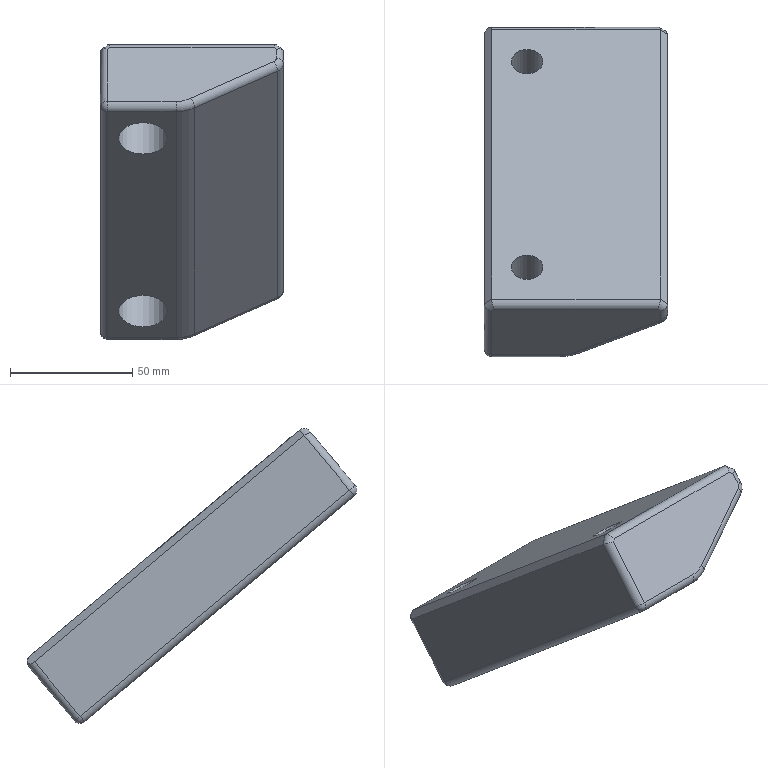Part | NX | features MAIN_BODY 2 | 1 solid | 37 faces | box 75 x 134.951 x 120.777 mm | volume 305128 mm3 | cylinder 20 | plane 11 | torus 4 | sphere 2 | commonest cylinder face diameters 6 x14 13 x2 20 x2 10 x1 30 x1
STEP:
#1=CARTESIAN_POINT('',(-217.5,186.664,-117.468));
#2=VERTEX_POINT('',#1);
#3=CARTESIAN_POINT('',(-217.5,191.644,-121.646));
#4=DIRECTION('',(0.,0.6428,0.766));
#5=DIRECTION('',(0.,-0.766,0.6428));
#6=AXIS2_PLACEMENT_3D('',#3,#4,#5);
#7=CIRCLE('',#6,6.5);
#8=EDGE_CURVE('',#2,#2,#7,.T.);
#9=ORIENTED_EDGE('',*,*,#8,.T.);
#10=EDGE_LOOP('',(#9));
#11=FACE_BOUND('',#10,.T.);
#12=CARTESIAN_POINT('',(-217.5,183.983,-115.218));
#13=VERTEX_POINT('',#12);
#14=CARTESIAN_POINT('',(-217.5,191.644,-121.646));
#15=DIRECTION('',(0.,0.6428,0.766));
#16=DIRECTION('',(0.,-0.766,0.6428));
#17=AXIS2_PLACEMENT_3D('',#14,#15,#16);
#18=CIRCLE('',#17,10.);
#19=EDGE_CURVE('',#13,#13,#18,.T.);
#20=ORIENTED_EDGE('',*,*,#19,.F.);
#21=EDGE_LOOP('',(#20));
#22=FACE_BOUND('',#21,.T.);
#23=CARTESIAN_POINT('',(-217.5,191.644,-121.646));
#24=DIRECTION('',(0.,0.6428,0.766));
#25=DIRECTION('',(0.,-0.766,0.6428));
#26=AXIS2_PLACEMENT_3D('',#23,#24,#25);
#27=PLANE('',#26);
#28=ADVANCED_FACE('',(#11,#22),#27,.F.);
#29=CARTESIAN_POINT('',(-163.,183.237,-100.55));
#30=VERTEX_POINT('',#29);
#31=CARTESIAN_POINT('',(-164.243,184.036,-99.598));
#32=VERTEX_POINT('',#31);
#33=CARTESIAN_POINT('',(-133.621,164.353,-123.055));
#34=DIRECTION('',(-0.7071,0.4545,0.5417));
#35=VECTOR('',#34,1000.);
#36=LINE('',#33,#35);
#37=EDGE_CURVE('',#30,#32,#36,.T.);
#38=ORIENTED_EDGE('',*,*,#37,.T.);
#39=CARTESIAN_POINT('',(-230.757,184.036,-99.598));
#40=VERTEX_POINT('',#39);
#41=CARTESIAN_POINT('',(-135.,184.036,-99.598));
#42=DIRECTION('',(-1.,0.,0.));
#43=VECTOR('',#42,1000.);
#44=LINE('',#41,#43);
#45=EDGE_CURVE('',#32,#40,#44,.T.);
#46=ORIENTED_EDGE('',*,*,#45,.T.);
#47=CARTESIAN_POINT('',(-232.,183.237,-100.55));
#48=VERTEX_POINT('',#47);
#49=CARTESIAN_POINT('',(-198.879,204.527,-75.177));
#50=DIRECTION('',(0.7071,0.4545,0.5417));
#51=VECTOR('',#50,1000.);
#52=LINE('',#49,#51);
#53=EDGE_CURVE('',#40,#48,#52,.F.);
#54=ORIENTED_EDGE('',*,*,#53,.T.);
#55=CARTESIAN_POINT('',(-232.,165.395,-121.813));
#56=VERTEX_POINT('',#55);
#57=CARTESIAN_POINT('',(-232.,163.467,-124.111));
#58=DIRECTION('',(0.,-0.6428,-0.766));
#59=VECTOR('',#58,1000.);
#60=LINE('',#57,#59);
#61=EDGE_CURVE('',#48,#56,#60,.T.);
#62=ORIENTED_EDGE('',*,*,#61,.T.);
#63=CARTESIAN_POINT('',(-204.019,165.395,-121.813));
#64=VERTEX_POINT('',#63);
#65=CARTESIAN_POINT('',(-135.,165.395,-121.813));
#66=DIRECTION('',(-1.,0.,0.));
#67=VECTOR('',#66,1000.);
#68=LINE('',#65,#67);
#69=EDGE_CURVE('',#56,#64,#68,.F.);
#70=ORIENTED_EDGE('',*,*,#69,.T.);
#71=CARTESIAN_POINT('',(-198.019,166.429,-120.581));
#72=VERTEX_POINT('',#71);
#73=CARTESIAN_POINT('',(-204.019,173.109,-112.62));
#74=DIRECTION('',(0.,-0.766,0.6428));
#75=DIRECTION('',(0.,-0.6428,-0.766));
#76=AXIS2_PLACEMENT_3D('',#73,#74,#75);
#77=CIRCLE('',#76,12.);
#78=EDGE_CURVE('',#64,#72,#77,.T.);
#79=ORIENTED_EDGE('',*,*,#78,.T.);
#80=CARTESIAN_POINT('',(-164.,179.054,-105.535));
#81=VERTEX_POINT('',#80);
#82=CARTESIAN_POINT('',(-152.75,183.229,-100.56));
#83=DIRECTION('',(0.866,0.3214,0.383));
#84=VECTOR('',#83,1000.);
#85=LINE('',#82,#84);
#86=EDGE_CURVE('',#72,#81,#85,.T.);
#87=ORIENTED_EDGE('',*,*,#86,.T.);
#88=CARTESIAN_POINT('',(-163.,180.167,-104.209));
#89=VERTEX_POINT('',#88);
#90=CARTESIAN_POINT('',(-165.,180.167,-104.209));
#91=DIRECTION('',(0.,-0.766,0.6428));
#92=DIRECTION('',(0.,-0.6428,-0.766));
#93=AXIS2_PLACEMENT_3D('',#90,#91,#92);
#94=CIRCLE('',#93,2.);
#95=EDGE_CURVE('',#81,#89,#94,.T.);
#96=ORIENTED_EDGE('',*,*,#95,.T.);
#97=CARTESIAN_POINT('',(-163.,184.036,-99.598));
#98=DIRECTION('',(0.,0.6428,0.766));
#99=VECTOR('',#98,1000.);
#100=LINE('',#97,#99);
#101=EDGE_CURVE('',#89,#30,#100,.T.);
#102=ORIENTED_EDGE('',*,*,#101,.T.);
#103=EDGE_LOOP('',(#38,#46,#54,#62,#70,#79,#87,#96,#102));
#104=FACE_BOUND('',#103,.T.);
#105=CARTESIAN_POINT('',(-135.,163.467,-124.111));
#106=DIRECTION('',(0.,-0.766,0.6428));
#107=DIRECTION('',(-1.,0.,0.));
#108=AXIS2_PLACEMENT_3D('',#105,#106,#107);
#109=PLANE('',#108);
#110=ADVANCED_FACE('',(#104),#109,.T.);
#111=CARTESIAN_POINT('',(-160.,182.465,-106.137));
#112=VERTEX_POINT('',#111);
#113=CARTESIAN_POINT('',(-163.,182.465,-106.137));
#114=DIRECTION('',(0.,-0.6428,-0.766));
#115=DIRECTION('',(0.,0.766,-0.6428));
#116=AXIS2_PLACEMENT_3D('',#113,#114,#115);
#117=CIRCLE('',#116,3.);
#118=EDGE_CURVE('',#112,#89,#117,.T.);
#119=ORIENTED_EDGE('',*,*,#118,.F.);
#120=CARTESIAN_POINT('',(-160.,186.334,-101.526));
#121=VERTEX_POINT('',#120);
#122=CARTESIAN_POINT('',(-160.,182.465,-106.137));
#123=DIRECTION('',(0.,0.6428,0.766));
#124=VECTOR('',#123,1000.);
#125=LINE('',#122,#124);
#126=EDGE_CURVE('',#121,#112,#125,.F.);
#127=ORIENTED_EDGE('',*,*,#126,.F.);
#128=CARTESIAN_POINT('',(-163.,185.536,-102.478));
#129=DIRECTION('',(0.3827,-0.5939,-0.7077));
#130=DIRECTION('',(-0.9239,-0.246,-0.2932));
#131=AXIS2_PLACEMENT_3D('',#128,#129,#130);
#132=ELLIPSE('',#131,3.247,3.);
#133=EDGE_CURVE('',#30,#121,#132,.F.);
#134=ORIENTED_EDGE('',*,*,#133,.F.);
#135=ORIENTED_EDGE('',*,*,#101,.F.);
#136=EDGE_LOOP('',(#119,#127,#134,#135));
#137=FACE_BOUND('',#136,.T.);
#138=CARTESIAN_POINT('',(-163.,165.765,-126.039));
#139=DIRECTION('',(0.,-0.6428,-0.766));
#140=DIRECTION('',(0.,0.766,-0.6428));
#141=AXIS2_PLACEMENT_3D('',#138,#139,#140);
#142=CYLINDRICAL_SURFACE('',#141,3.);
#143=ADVANCED_FACE('',(#137),#142,.T.);
#144=CARTESIAN_POINT('',(-204.019,165.765,-126.039));
#145=VERTEX_POINT('',#144);
#146=CARTESIAN_POINT('',(-204.019,167.693,-123.741));
#147=DIRECTION('',(-1.,0.,0.));
#148=DIRECTION('',(0.,0.9063,0.4226));
#149=AXIS2_PLACEMENT_3D('',#146,#147,#148);
#150=CIRCLE('',#149,3.);
#151=EDGE_CURVE('',#145,#64,#150,.T.);
#152=ORIENTED_EDGE('',*,*,#151,.T.);
#153=ORIENTED_EDGE('',*,*,#69,.F.);
#154=CARTESIAN_POINT('',(-232.,165.765,-126.039));
#155=VERTEX_POINT('',#154);
#156=CARTESIAN_POINT('',(-232.,167.693,-123.741));
#157=DIRECTION('',(-1.,0.,0.));
#158=DIRECTION('',(0.,0.9063,0.4226));
#159=AXIS2_PLACEMENT_3D('',#156,#157,#158);
#160=CIRCLE('',#159,3.);
#161=EDGE_CURVE('',#155,#56,#160,.T.);
#162=ORIENTED_EDGE('',*,*,#161,.F.);
#163=CARTESIAN_POINT('',(-285.,165.765,-126.039));
#164=DIRECTION('',(-1.,0.,0.));
#165=VECTOR('',#164,1000.);
#166=LINE('',#163,#165);
#167=EDGE_CURVE('',#145,#155,#166,.T.);
#168=ORIENTED_EDGE('',*,*,#167,.F.);
#169=EDGE_LOOP('',(#152,#153,#162,#168));
#170=FACE_BOUND('',#169,.T.);
#171=CARTESIAN_POINT('',(-285.,167.693,-123.741));
#172=DIRECTION('',(-1.,0.,0.));
#173=DIRECTION('',(0.,0.4226,-0.9063));
#174=AXIS2_PLACEMENT_3D('',#171,#172,#173);
#175=CYLINDRICAL_SURFACE('',#174,3.);
#176=ADVANCED_FACE('',(#170),#175,.T.);
#177=ORIENTED_EDGE('',*,*,#19,.T.);
#178=EDGE_LOOP('',(#177));
#179=FACE_BOUND('',#178,.T.);
#180=CARTESIAN_POINT('',(-217.5,171.127,-130.539));
#181=VERTEX_POINT('',#180);
#182=CARTESIAN_POINT('',(-217.5,178.788,-136.967));
#183=DIRECTION('',(0.,0.6428,0.766));
#184=DIRECTION('',(0.,-0.766,0.6428));
#185=AXIS2_PLACEMENT_3D('',#182,#183,#184);
#186=CIRCLE('',#185,10.);
#187=EDGE_CURVE('',#181,#181,#186,.T.);
#188=ORIENTED_EDGE('',*,*,#187,.F.);
#189=EDGE_LOOP('',(#188));
#190=FACE_BOUND('',#189,.T.);
#191=CARTESIAN_POINT('',(-217.5,178.788,-136.967));
#192=DIRECTION('',(0.,0.6428,0.766));
#193=DIRECTION('',(0.,-0.766,0.6428));
#194=AXIS2_PLACEMENT_3D('',#191,#192,#193);
#195=CYLINDRICAL_SURFACE('',#194,10.);
#196=ADVANCED_FACE('',(#179,#190),#195,.F.);
#197=CARTESIAN_POINT('',(-163.,188.263,-99.228));
#198=VERTEX_POINT('',#197);
#199=CARTESIAN_POINT('',(-164.243,186.334,-101.526));
#200=DIRECTION('',(-0.9239,0.246,0.2932));
#201=DIRECTION('',(-0.3827,-0.5939,-0.7077));
#202=AXIS2_PLACEMENT_3D('',#199,#200,#201);
#203=ELLIPSE('',#202,3.247,3.);
#204=EDGE_CURVE('',#32,#198,#203,.T.);
#205=ORIENTED_EDGE('',*,*,#204,.T.);
#206=CARTESIAN_POINT('',(-232.,188.263,-99.228));
#207=VERTEX_POINT('',#206);
#208=CARTESIAN_POINT('',(-135.,188.263,-99.228));
#209=DIRECTION('',(-1.,0.,0.));
#210=VECTOR('',#209,1000.);
#211=LINE('',#208,#210);
#212=EDGE_CURVE('',#207,#198,#211,.F.);
#213=ORIENTED_EDGE('',*,*,#212,.F.);
#214=CARTESIAN_POINT('',(-230.757,186.334,-101.526));
#215=DIRECTION('',(-0.9239,-0.246,-0.2932));
#216=DIRECTION('',(-0.3827,0.5939,0.7077));
#217=AXIS2_PLACEMENT_3D('',#214,#215,#216);
#218=ELLIPSE('',#217,3.247,3.);
#219=EDGE_CURVE('',#40,#207,#218,.T.);
#220=ORIENTED_EDGE('',*,*,#219,.F.);
#221=ORIENTED_EDGE('',*,*,#45,.F.);
#222=EDGE_LOOP('',(#205,#213,#220,#221));
#223=FACE_BOUND('',#222,.T.);
#224=CARTESIAN_POINT('',(-135.,186.334,-101.526));
#225=DIRECTION('',(-1.,0.,0.));
#226=DIRECTION('',(0.,0.4226,-0.9063));
#227=AXIS2_PLACEMENT_3D('',#224,#225,#226);
#228=CYLINDRICAL_SURFACE('',#227,3.);
#229=ADVANCED_FACE('',(#223),#228,.T.);
#230=CARTESIAN_POINT('',(-217.5,196.306,-105.977));
#231=VERTEX_POINT('',#230);
#232=CARTESIAN_POINT('',(-217.5,201.285,-110.155));
#233=DIRECTION('',(0.,0.6428,0.766));
#234=DIRECTION('',(0.,-0.766,0.6428));
#235=AXIS2_PLACEMENT_3D('',#232,#233,#234);
#236=CIRCLE('',#235,6.5);
#237=EDGE_CURVE('',#231,#231,#236,.T.);
#238=ORIENTED_EDGE('',*,*,#237,.T.);
#239=EDGE_LOOP('',(#238));
#240=FACE_BOUND('',#239,.T.);
#241=ORIENTED_EDGE('',*,*,#8,.F.);
#242=EDGE_LOOP('',(#241));
#243=FACE_BOUND('',#242,.T.);
#244=CARTESIAN_POINT('',(-217.5,191.644,-121.646));
#245=DIRECTION('',(0.,0.6428,0.766));
#246=DIRECTION('',(0.,-0.766,0.6428));
#247=AXIS2_PLACEMENT_3D('',#244,#245,#246);
#248=CYLINDRICAL_SURFACE('',#247,6.5);
#249=ADVANCED_FACE('',(#240,#243),#248,.F.);
#250=CARTESIAN_POINT('',(-235.,186.334,-101.526));
#251=VERTEX_POINT('',#250);
#252=CARTESIAN_POINT('',(-232.,185.536,-102.478));
#253=DIRECTION('',(-0.3827,-0.5939,-0.7077));
#254=DIRECTION('',(0.9239,-0.246,-0.2932));
#255=AXIS2_PLACEMENT_3D('',#252,#253,#254);
#256=ELLIPSE('',#255,3.247,3.);
#257=EDGE_CURVE('',#48,#251,#256,.T.);
#258=ORIENTED_EDGE('',*,*,#257,.T.);
#259=CARTESIAN_POINT('',(-235.,167.693,-123.741));
#260=VERTEX_POINT('',#259);
#261=CARTESIAN_POINT('',(-235.,194.691,-91.567));
#262=DIRECTION('',(0.,-0.6428,-0.766));
#263=VECTOR('',#262,1000.);
#264=LINE('',#261,#263);
#265=EDGE_CURVE('',#260,#251,#264,.F.);
#266=ORIENTED_EDGE('',*,*,#265,.F.);
#267=CARTESIAN_POINT('',(-232.,167.693,-123.741));
#268=DIRECTION('',(0.,-0.6428,-0.766));
#269=DIRECTION('',(0.,0.766,-0.6428));
#270=AXIS2_PLACEMENT_3D('',#267,#268,#269);
#271=CIRCLE('',#270,3.);
#272=EDGE_CURVE('',#56,#260,#271,.T.);
#273=ORIENTED_EDGE('',*,*,#272,.F.);
#274=ORIENTED_EDGE('',*,*,#61,.F.);
#275=EDGE_LOOP('',(#258,#266,#273,#274));
#276=FACE_BOUND('',#275,.T.);
#277=CARTESIAN_POINT('',(-232.,165.765,-126.039));
#278=DIRECTION('',(0.,-0.6428,-0.766));
#279=DIRECTION('',(0.,0.766,-0.6428));
#280=AXIS2_PLACEMENT_3D('',#277,#278,#279);
#281=CYLINDRICAL_SURFACE('',#280,3.);
#282=ADVANCED_FACE('',(#276),#281,.T.);
#283=CARTESIAN_POINT('',(-162.5,179.682,-109.454));
#284=VERTEX_POINT('',#283);
#285=CARTESIAN_POINT('',(-164.,181.352,-107.464));
#286=DIRECTION('',(-0.866,-0.3214,-0.383));
#287=DIRECTION('',(-0.4636,0.803,0.3745));
#288=AXIS2_PLACEMENT_3D('',#285,#286,#287);
#289=CIRCLE('',#288,3.);
#290=EDGE_CURVE('',#284,#81,#289,.T.);
#291=ORIENTED_EDGE('',*,*,#290,.T.);
#292=ORIENTED_EDGE('',*,*,#86,.F.);
#293=CARTESIAN_POINT('',(-196.519,167.057,-124.5));
#294=VERTEX_POINT('',#293);
#295=CARTESIAN_POINT('',(-198.019,168.727,-122.51));
#296=DIRECTION('',(-0.866,-0.3214,-0.383));
#297=DIRECTION('',(-0.4636,0.803,0.3745));
#298=AXIS2_PLACEMENT_3D('',#295,#296,#297);
#299=CIRCLE('',#298,3.);
#300=EDGE_CURVE('',#294,#72,#299,.T.);
#301=ORIENTED_EDGE('',*,*,#300,.F.);
#302=CARTESIAN_POINT('',(-200.,165.765,-126.039));
#303=DIRECTION('',(0.866,0.3214,0.383));
#304=VECTOR('',#303,1000.);
#305=LINE('',#302,#304);
#306=EDGE_CURVE('',#284,#294,#305,.F.);
#307=ORIENTED_EDGE('',*,*,#306,.F.);
#308=EDGE_LOOP('',(#291,#292,#301,#307));
#309=FACE_BOUND('',#308,.T.);
#310=CARTESIAN_POINT('',(-152.75,185.527,-102.488));
#311=DIRECTION('',(0.866,0.3214,0.383));
#312=DIRECTION('',(0.4636,-0.803,-0.3745));
#313=AXIS2_PLACEMENT_3D('',#310,#311,#312);
#314=CYLINDRICAL_SURFACE('',#313,3.);
#315=ADVANCED_FACE('',(#309),#314,.T.);
#316=ORIENTED_EDGE('',*,*,#219,.T.);
#317=CARTESIAN_POINT('',(-232.,188.263,-99.228));
#318=DIRECTION('',(-0.7071,-0.4545,-0.5417));
#319=VECTOR('',#318,1000.);
#320=LINE('',#317,#319);
#321=EDGE_CURVE('',#251,#207,#320,.F.);
#322=ORIENTED_EDGE('',*,*,#321,.F.);
#323=ORIENTED_EDGE('',*,*,#257,.F.);
#324=ORIENTED_EDGE('',*,*,#53,.F.);
#325=EDGE_LOOP('',(#316,#322,#323,#324));
#326=FACE_BOUND('',#325,.T.);
#327=CARTESIAN_POINT('',(-198.879,206.826,-77.105));
#328=DIRECTION('',(0.7071,0.4545,0.5417));
#329=DIRECTION('',(0.6715,-0.6715,-0.3131));
#330=AXIS2_PLACEMENT_3D('',#327,#328,#329);
#331=CYLINDRICAL_SURFACE('',#330,3.);
#332=ADVANCED_FACE('',(#326),#331,.T.);
#333=ORIENTED_EDGE('',*,*,#133,.T.);
#334=CARTESIAN_POINT('',(-160.,186.334,-101.526));
#335=DIRECTION('',(-0.7071,0.4545,0.5417));
#336=VECTOR('',#335,1000.);
#337=LINE('',#334,#336);
#338=EDGE_CURVE('',#198,#121,#337,.F.);
#339=ORIENTED_EDGE('',*,*,#338,.F.);
#340=ORIENTED_EDGE('',*,*,#204,.F.);
#341=ORIENTED_EDGE('',*,*,#37,.F.);
#342=EDGE_LOOP('',(#333,#339,#340,#341));
#343=FACE_BOUND('',#342,.T.);
#344=CARTESIAN_POINT('',(-133.621,166.651,-124.983));
#345=DIRECTION('',(-0.7071,0.4545,0.5417));
#346=DIRECTION('',(0.6715,0.6715,0.3131));
#347=AXIS2_PLACEMENT_3D('',#344,#345,#346);
#348=CYLINDRICAL_SURFACE('',#347,3.);
#349=ADVANCED_FACE('',(#343),#348,.T.);
#350=ORIENTED_EDGE('',*,*,#118,.T.);
#351=ORIENTED_EDGE('',*,*,#95,.F.);
#352=ORIENTED_EDGE('',*,*,#290,.F.);
#353=CARTESIAN_POINT('',(-165.,182.465,-106.137));
#354=DIRECTION('',(0.,-0.766,0.6428));
#355=DIRECTION('',(0.,-0.6428,-0.766));
#356=AXIS2_PLACEMENT_3D('',#353,#354,#355);
#357=CIRCLE('',#356,5.);
#358=EDGE_CURVE('',#112,#284,#357,.F.);
#359=ORIENTED_EDGE('',*,*,#358,.F.);
#360=EDGE_LOOP('',(#350,#351,#352,#359));
#361=FACE_BOUND('',#360,.T.);
#362=CARTESIAN_POINT('',(-165.,182.465,-106.137));
#363=DIRECTION('',(0.,-0.766,0.6428));
#364=DIRECTION('',(0.,-0.6428,-0.766));
#365=AXIS2_PLACEMENT_3D('',#362,#363,#364);
#366=DEGENERATE_TOROIDAL_SURFACE('',#365,2.,3.,.T.);
#367=ADVANCED_FACE('',(#361),#366,.T.);
#368=ORIENTED_EDGE('',*,*,#300,.T.);
#369=ORIENTED_EDGE('',*,*,#78,.F.);
#370=ORIENTED_EDGE('',*,*,#151,.F.);
#371=CARTESIAN_POINT('',(-204.019,175.407,-114.549));
#372=DIRECTION('',(0.,-0.766,0.6428));
#373=DIRECTION('',(0.,-0.6428,-0.766));
#374=AXIS2_PLACEMENT_3D('',#371,#372,#373);
#375=CIRCLE('',#374,15.);
#376=EDGE_CURVE('',#294,#145,#375,.F.);
#377=ORIENTED_EDGE('',*,*,#376,.F.);
#378=EDGE_LOOP('',(#368,#369,#370,#377));
#379=FACE_BOUND('',#378,.T.);
#380=CARTESIAN_POINT('',(-204.019,175.407,-114.549));
#381=DIRECTION('',(0.,-0.766,0.6428));
#382=DIRECTION('',(0.,-0.6428,-0.766));
#383=AXIS2_PLACEMENT_3D('',#380,#381,#382);
#384=TOROIDAL_SURFACE('',#383,12.,3.);
#385=ADVANCED_FACE('',(#379),#384,.T.);
#386=ORIENTED_EDGE('',*,*,#161,.T.);
#387=ORIENTED_EDGE('',*,*,#272,.T.);
#388=CARTESIAN_POINT('',(-232.,167.693,-123.741));
#389=DIRECTION('',(0.,-0.766,0.6428));
#390=DIRECTION('',(0.,-0.6428,-0.766));
#391=AXIS2_PLACEMENT_3D('',#388,#389,#390);
#392=CIRCLE('',#391,3.);
#393=EDGE_CURVE('',#155,#260,#392,.F.);
#394=ORIENTED_EDGE('',*,*,#393,.F.);
#395=EDGE_LOOP('',(#386,#387,#394));
#396=FACE_BOUND('',#395,.T.);
#397=CARTESIAN_POINT('',(-232.,167.693,-123.741));
#398=DIRECTION('',(0.,-0.9063,-0.4226));
#399=DIRECTION('',(0.,0.4226,-0.9063));
#400=AXIS2_PLACEMENT_3D('',#397,#398,#399);
#401=SPHERICAL_SURFACE('',#400,3.);
#402=ADVANCED_FACE('',(#396),#401,.T.);
#403=CARTESIAN_POINT('',(-162.5,289.992,-202.015));
#404=VERTEX_POINT('',#403);
#405=CARTESIAN_POINT('',(-160.,292.776,-198.698));
#406=VERTEX_POINT('',#405);
#407=CARTESIAN_POINT('',(-165.,292.776,-198.698));
#408=DIRECTION('',(0.,-0.766,0.6428));
#409=DIRECTION('',(0.,-0.6428,-0.766));
#410=AXIS2_PLACEMENT_3D('',#407,#408,#409);
#411=CIRCLE('',#410,5.);
#412=EDGE_CURVE('',#404,#406,#411,.T.);
#413=ORIENTED_EDGE('',*,*,#412,.T.);
#414=CARTESIAN_POINT('',(-160.,295.074,-200.627));
#415=DIRECTION('',(0.,-0.766,0.6428));
#416=VECTOR('',#415,1000.);
#417=LINE('',#414,#416);
#418=EDGE_CURVE('',#112,#406,#417,.F.);
#419=ORIENTED_EDGE('',*,*,#418,.F.);
#420=ORIENTED_EDGE('',*,*,#358,.T.);
#421=CARTESIAN_POINT('',(-162.5,177.384,-107.526));
#422=DIRECTION('',(0.,-0.766,0.6428));
#423=VECTOR('',#422,1000.);
#424=LINE('',#421,#423);
#425=EDGE_CURVE('',#404,#284,#424,.T.);
#426=ORIENTED_EDGE('',*,*,#425,.F.);
#427=EDGE_LOOP('',(#413,#419,#420,#426));
#428=FACE_BOUND('',#427,.T.);
#429=CARTESIAN_POINT('',(-165.,180.167,-104.209));
#430=DIRECTION('',(0.,0.766,-0.6428));
#431=DIRECTION('',(0.,0.6428,0.766));
#432=AXIS2_PLACEMENT_3D('',#429,#430,#431);
#433=CYLINDRICAL_SURFACE('',#432,5.);
#434=ADVANCED_FACE('',(#428),#433,.T.);
#435=CARTESIAN_POINT('',(-204.019,276.076,-218.601));
#436=VERTEX_POINT('',#435);
#437=CARTESIAN_POINT('',(-196.519,277.367,-217.061));
#438=VERTEX_POINT('',#437);
#439=CARTESIAN_POINT('',(-204.019,285.717,-207.11));
#440=DIRECTION('',(0.,-0.766,0.6428));
#441=DIRECTION('',(0.,-0.6428,-0.766));
#442=AXIS2_PLACEMENT_3D('',#439,#440,#441);
#443=CIRCLE('',#442,15.);
#444=EDGE_CURVE('',#436,#438,#443,.T.);
#445=ORIENTED_EDGE('',*,*,#444,.T.);
#446=CARTESIAN_POINT('',(-196.519,164.759,-122.572));
#447=DIRECTION('',(0.,0.766,-0.6428));
#448=VECTOR('',#447,1000.);
#449=LINE('',#446,#448);
#450=EDGE_CURVE('',#294,#438,#449,.T.);
#451=ORIENTED_EDGE('',*,*,#450,.F.);
#452=ORIENTED_EDGE('',*,*,#376,.T.);
#453=CARTESIAN_POINT('',(-204.019,52.391,-30.907));
#454=DIRECTION('',(0.,0.766,-0.6428));
#455=VECTOR('',#454,1000.);
#456=LINE('',#453,#455);
#457=EDGE_CURVE('',#436,#145,#456,.F.);
#458=ORIENTED_EDGE('',*,*,#457,.F.);
#459=EDGE_LOOP('',(#445,#451,#452,#458));
#460=FACE_BOUND('',#459,.T.);
#461=CARTESIAN_POINT('',(-204.019,173.109,-112.62));
#462=DIRECTION('',(0.,0.766,-0.6428));
#463=DIRECTION('',(0.,0.6428,0.766));
#464=AXIS2_PLACEMENT_3D('',#461,#462,#463);
#465=CYLINDRICAL_SURFACE('',#464,15.);
#466=ADVANCED_FACE('',(#460),#465,.T.);
#467=ORIENTED_EDGE('',*,*,#425,.T.);
#468=ORIENTED_EDGE('',*,*,#306,.T.);
#469=ORIENTED_EDGE('',*,*,#450,.T.);
#470=CARTESIAN_POINT('',(-162.5,289.992,-202.015));
#471=DIRECTION('',(0.866,0.3214,0.383));
#472=VECTOR('',#471,1000.);
#473=LINE('',#470,#472);
#474=EDGE_CURVE('',#438,#404,#473,.T.);
#475=ORIENTED_EDGE('',*,*,#474,.T.);
#476=EDGE_LOOP('',(#467,#468,#469,#475));
#477=FACE_BOUND('',#476,.T.);
#478=CARTESIAN_POINT('',(-200.,163.467,-124.111));
#479=DIRECTION('',(0.5,-0.5567,-0.6634));
#480=DIRECTION('',(0.,0.766,-0.6428));
#481=AXIS2_PLACEMENT_3D('',#478,#479,#480);
#482=PLANE('',#481);
#483=ADVANCED_FACE('',(#477),#482,.T.);
#484=CARTESIAN_POINT('',(-232.,276.076,-218.601));
#485=VERTEX_POINT('',#484);
#486=CARTESIAN_POINT('',(-235.,278.004,-216.303));
#487=VERTEX_POINT('',#486);
#488=CARTESIAN_POINT('',(-232.,278.004,-216.303));
#489=DIRECTION('',(0.,0.766,-0.6428));
#490=DIRECTION('',(0.,0.6428,0.766));
#491=AXIS2_PLACEMENT_3D('',#488,#489,#490);
#492=CIRCLE('',#491,3.);
#493=EDGE_CURVE('',#485,#487,#492,.T.);
#494=ORIENTED_EDGE('',*,*,#493,.F.);
#495=CARTESIAN_POINT('',(-232.,52.391,-30.907));
#496=DIRECTION('',(0.,0.766,-0.6428));
#497=VECTOR('',#496,1000.);
#498=LINE('',#495,#497);
#499=EDGE_CURVE('',#155,#485,#498,.T.);
#500=ORIENTED_EDGE('',*,*,#499,.F.);
#501=ORIENTED_EDGE('',*,*,#393,.T.);
#502=CARTESIAN_POINT('',(-235.,54.319,-28.609));
#503=DIRECTION('',(0.,0.766,-0.6428));
#504=VECTOR('',#503,1000.);
#505=LINE('',#502,#504);
#506=EDGE_CURVE('',#487,#260,#505,.F.);
#507=ORIENTED_EDGE('',*,*,#506,.F.);
#508=EDGE_LOOP('',(#494,#500,#501,#507));
#509=FACE_BOUND('',#508,.T.);
#510=CARTESIAN_POINT('',(-232.,54.319,-28.609));
#511=DIRECTION('',(0.,0.766,-0.6428));
#512=DIRECTION('',(0.,0.6428,0.766));
#513=AXIS2_PLACEMENT_3D('',#510,#511,#512);
#514=CYLINDRICAL_SURFACE('',#513,3.);
#515=ADVANCED_FACE('',(#509),#514,.T.);
#516=CARTESIAN_POINT('',(-233.5,299.599,-194.608));
#517=VERTEX_POINT('',#516);
#518=CARTESIAN_POINT('',(-235.,296.645,-194.087));
#519=VERTEX_POINT('',#518);
#520=CARTESIAN_POINT('',(-232.,298.573,-191.789));
#521=DIRECTION('',(0.7071,-0.4545,-0.5417));
#522=DIRECTION('',(0.7071,0.4545,0.5417));
#523=AXIS2_PLACEMENT_3D('',#520,#521,#522);
#524=ELLIPSE('',#523,4.243,3.);
#525=EDGE_CURVE('',#517,#519,#524,.F.);
#526=ORIENTED_EDGE('',*,*,#525,.T.);
#527=CARTESIAN_POINT('',(-235.,72.96,-6.393));
#528=DIRECTION('',(0.,0.766,-0.6428));
#529=VECTOR('',#528,1000.);
#530=LINE('',#527,#529);
#531=EDGE_CURVE('',#251,#519,#530,.T.);
#532=ORIENTED_EDGE('',*,*,#531,.F.);
#533=ORIENTED_EDGE('',*,*,#321,.T.);
#534=CARTESIAN_POINT('',(-232.,298.573,-191.789));
#535=VERTEX_POINT('',#534);
#536=CARTESIAN_POINT('',(-232.,74.888,-4.095));
#537=DIRECTION('',(0.,0.766,-0.6428));
#538=VECTOR('',#537,1000.);
#539=LINE('',#536,#538);
#540=EDGE_CURVE('',#207,#535,#539,.T.);
#541=ORIENTED_EDGE('',*,*,#540,.T.);
#542=CARTESIAN_POINT('',(-235.,296.645,-194.087));
#543=DIRECTION('',(0.7071,-0.4545,-0.5417));
#544=DIRECTION('',(-0.7071,-0.4545,-0.5417));
#545=AXIS2_PLACEMENT_3D('',#542,#543,#544);
#546=ELLIPSE('',#545,4.243,3.);
#547=EDGE_CURVE('',#535,#517,#546,.F.);
#548=ORIENTED_EDGE('',*,*,#547,.T.);
#549=EDGE_LOOP('',(#526,#532,#533,#541,#548));
#550=FACE_BOUND('',#549,.T.);
#551=CARTESIAN_POINT('',(-232.,74.888,-4.095));
#552=DIRECTION('',(0.7071,-0.4545,-0.5417));
#553=DIRECTION('',(-0.6715,-0.6715,-0.3131));
#554=AXIS2_PLACEMENT_3D('',#551,#552,#553);
#555=PLANE('',#554);
#556=ADVANCED_FACE('',(#550),#555,.F.);
#557=ORIENTED_EDGE('',*,*,#506,.T.);
#558=ORIENTED_EDGE('',*,*,#265,.T.);
#559=ORIENTED_EDGE('',*,*,#531,.T.);
#560=CARTESIAN_POINT('',(-235.,276.076,-218.601));
#561=DIRECTION('',(0.,-0.6428,-0.766));
#562=VECTOR('',#561,1000.);
#563=LINE('',#560,#562);
#564=EDGE_CURVE('',#519,#487,#563,.T.);
#565=ORIENTED_EDGE('',*,*,#564,.T.);
#566=EDGE_LOOP('',(#557,#558,#559,#565));
#567=FACE_BOUND('',#566,.T.);
#568=CARTESIAN_POINT('',(-235.,81.316,3.565));
#569=DIRECTION('',(-1.,0.,0.));
#570=DIRECTION('',(0.,0.766,-0.6428));
#571=AXIS2_PLACEMENT_3D('',#568,#569,#570);
#572=PLANE('',#571);
#573=ADVANCED_FACE('',(#567),#572,.T.);
#574=CARTESIAN_POINT('',(-160.,296.645,-194.087));
#575=VERTEX_POINT('',#574);
#576=CARTESIAN_POINT('',(-163.,298.573,-191.789));
#577=VERTEX_POINT('',#576);
#578=CARTESIAN_POINT('',(-163.,298.573,-191.789));
#579=DIRECTION('',(0.7071,-0.4545,-0.5417));
#580=VECTOR('',#579,1000.);
#581=LINE('',#578,#580);
#582=EDGE_CURVE('',#575,#577,#581,.F.);
#583=ORIENTED_EDGE('',*,*,#582,.T.);
#584=CARTESIAN_POINT('',(-163.,300.871,-193.718));
#585=DIRECTION('',(0.,0.766,-0.6428));
#586=VECTOR('',#585,1000.);
#587=LINE('',#584,#586);
#588=EDGE_CURVE('',#198,#577,#587,.T.);
#589=ORIENTED_EDGE('',*,*,#588,.F.);
#590=ORIENTED_EDGE('',*,*,#338,.T.);
#591=CARTESIAN_POINT('',(-160.,184.036,-99.598));
#592=DIRECTION('',(0.,-0.766,0.6428));
#593=VECTOR('',#592,1000.);
#594=LINE('',#591,#593);
#595=EDGE_CURVE('',#575,#121,#594,.T.);
#596=ORIENTED_EDGE('',*,*,#595,.F.);
#597=EDGE_LOOP('',(#583,#589,#590,#596));
#598=FACE_BOUND('',#597,.T.);
#599=CARTESIAN_POINT('',(-160.,-1.347,55.957));
#600=DIRECTION('',(0.7071,0.4545,0.5417));
#601=DIRECTION('',(0.6715,-0.6715,-0.3131));
#602=AXIS2_PLACEMENT_3D('',#599,#600,#601);
#603=PLANE('',#602);
#604=ADVANCED_FACE('',(#598),#603,.T.);
#605=CARTESIAN_POINT('',(-232.,298.573,-191.789));
#606=DIRECTION('',(1.,0.,0.));
#607=VECTOR('',#606,1000.);
#608=LINE('',#605,#607);
#609=EDGE_CURVE('',#577,#535,#608,.F.);
#610=ORIENTED_EDGE('',*,*,#609,.T.);
#611=ORIENTED_EDGE('',*,*,#540,.F.);
#612=ORIENTED_EDGE('',*,*,#212,.T.);
#613=ORIENTED_EDGE('',*,*,#588,.T.);
#614=EDGE_LOOP('',(#610,#611,#612,#613));
#615=FACE_BOUND('',#614,.T.);
#616=ORIENTED_EDGE('',*,*,#237,.F.);
#617=EDGE_LOOP('',(#616));
#618=FACE_BOUND('',#617,.T.);
#619=CARTESIAN_POINT('',(-217.5,280.571,-176.684));
#620=VERTEX_POINT('',#619);
#621=CARTESIAN_POINT('',(-217.5,285.55,-180.862));
#622=DIRECTION('',(0.,0.6428,0.766));
#623=DIRECTION('',(0.,-0.766,0.6428));
#624=AXIS2_PLACEMENT_3D('',#621,#622,#623);
#625=CIRCLE('',#624,6.5);
#626=EDGE_CURVE('',#620,#620,#625,.T.);
#627=ORIENTED_EDGE('',*,*,#626,.F.);
#628=EDGE_LOOP('',(#627));
#629=FACE_BOUND('',#628,.T.);
#630=CARTESIAN_POINT('',(-135.,74.888,-4.095));
#631=DIRECTION('',(0.,0.6428,0.766));
#632=DIRECTION('',(1.,0.,0.));
#633=AXIS2_PLACEMENT_3D('',#630,#631,#632);
#634=PLANE('',#633);
#635=ADVANCED_FACE('',(#615,#618,#629),#634,.T.);
#636=ORIENTED_EDGE('',*,*,#457,.T.);
#637=ORIENTED_EDGE('',*,*,#167,.T.);
#638=ORIENTED_EDGE('',*,*,#499,.T.);
#639=CARTESIAN_POINT('',(-204.019,276.076,-218.601));
#640=DIRECTION('',(1.,0.,0.));
#641=VECTOR('',#640,1000.);
#642=LINE('',#639,#641);
#643=EDGE_CURVE('',#485,#436,#642,.T.);
#644=ORIENTED_EDGE('',*,*,#643,.T.);
#645=EDGE_LOOP('',(#636,#637,#638,#644));
#646=FACE_BOUND('',#645,.T.);
#647=ORIENTED_EDGE('',*,*,#187,.T.);
#648=EDGE_LOOP('',(#647));
#649=FACE_BOUND('',#648,.T.);
#650=CARTESIAN_POINT('',(-217.5,255.392,-201.246));
#651=VERTEX_POINT('',#650);
#652=CARTESIAN_POINT('',(-217.5,263.053,-207.673));
#653=DIRECTION('',(0.,0.6428,0.766));
#654=DIRECTION('',(0.,-0.766,0.6428));
#655=AXIS2_PLACEMENT_3D('',#652,#653,#654);
#656=CIRCLE('',#655,10.);
#657=EDGE_CURVE('',#651,#651,#656,.T.);
#658=ORIENTED_EDGE('',*,*,#657,.T.);
#659=EDGE_LOOP('',(#658));
#660=FACE_BOUND('',#659,.T.);
#661=CARTESIAN_POINT('',(-285.,52.391,-30.907));
#662=DIRECTION('',(0.,-0.6428,-0.766));
#663=DIRECTION('',(0.,0.766,-0.6428));
#664=AXIS2_PLACEMENT_3D('',#661,#662,#663);
#665=PLANE('',#664);
#666=ADVANCED_FACE('',(#646,#649,#660),#665,.T.);
#667=ORIENTED_EDGE('',*,*,#595,.T.);
#668=ORIENTED_EDGE('',*,*,#126,.T.);
#669=ORIENTED_EDGE('',*,*,#418,.T.);
#670=CARTESIAN_POINT('',(-160.,303.715,-185.661));
#671=DIRECTION('',(0.,0.6428,0.766));
#672=VECTOR('',#671,1000.);
#673=LINE('',#670,#672);
#674=EDGE_CURVE('',#406,#575,#673,.T.);
#675=ORIENTED_EDGE('',*,*,#674,.T.);
#676=EDGE_LOOP('',(#667,#668,#669,#675));
#677=FACE_BOUND('',#676,.T.);
#678=CARTESIAN_POINT('',(-160.,5.724,64.383));
#679=DIRECTION('',(-1.,0.,0.));
#680=DIRECTION('',(0.,-0.1736,0.9848));
#681=AXIS2_PLACEMENT_3D('',#678,#679,#680);
#682=PLANE('',#681);
#683=ADVANCED_FACE('',(#677),#682,.F.);
#684=CARTESIAN_POINT('',(-232.,298.943,-196.016));
#685=VERTEX_POINT('',#684);
#686=CARTESIAN_POINT('',(-164.243,298.943,-196.016));
#687=VERTEX_POINT('',#686);
#688=CARTESIAN_POINT('',(-163.,298.943,-196.016));
#689=DIRECTION('',(1.,0.,0.));
#690=VECTOR('',#689,1000.);
#691=LINE('',#688,#690);
#692=EDGE_CURVE('',#685,#687,#691,.T.);
#693=ORIENTED_EDGE('',*,*,#692,.T.);
#694=CARTESIAN_POINT('',(-163.,298.144,-196.968));
#695=VERTEX_POINT('',#694);
#696=CARTESIAN_POINT('',(-162.121,297.579,-197.641));
#697=DIRECTION('',(0.7071,-0.4545,-0.5417));
#698=VECTOR('',#697,1000.);
#699=LINE('',#696,#698);
#700=EDGE_CURVE('',#687,#695,#699,.T.);
#701=ORIENTED_EDGE('',*,*,#700,.T.);
#702=CARTESIAN_POINT('',(-163.,295.074,-200.627));
#703=VERTEX_POINT('',#702);
#704=CARTESIAN_POINT('',(-163.,278.374,-220.529));
#705=DIRECTION('',(0.,0.6428,0.766));
#706=VECTOR('',#705,1000.);
#707=LINE('',#704,#706);
#708=EDGE_CURVE('',#695,#703,#707,.F.);
#709=ORIENTED_EDGE('',*,*,#708,.T.);
#710=CARTESIAN_POINT('',(-164.,293.96,-201.954));
#711=VERTEX_POINT('',#710);
#712=CARTESIAN_POINT('',(-165.,295.074,-200.627));
#713=DIRECTION('',(0.,-0.766,0.6428));
#714=DIRECTION('',(0.,-0.6428,-0.766));
#715=AXIS2_PLACEMENT_3D('',#712,#713,#714);
#716=CIRCLE('',#715,2.);
#717=EDGE_CURVE('',#703,#711,#716,.F.);
#718=ORIENTED_EDGE('',*,*,#717,.T.);
#719=CARTESIAN_POINT('',(-198.019,281.335,-216.999));
#720=VERTEX_POINT('',#719);
#721=CARTESIAN_POINT('',(-198.019,281.335,-216.999));
#722=DIRECTION('',(0.866,0.3214,0.383));
#723=VECTOR('',#722,1000.);
#724=LINE('',#721,#723);
#725=EDGE_CURVE('',#711,#720,#724,.F.);
#726=ORIENTED_EDGE('',*,*,#725,.T.);
#727=CARTESIAN_POINT('',(-204.019,280.302,-218.231));
#728=VERTEX_POINT('',#727);
#729=CARTESIAN_POINT('',(-204.019,288.015,-209.038));
#730=DIRECTION('',(0.,-0.766,0.6428));
#731=DIRECTION('',(0.,-0.6428,-0.766));
#732=AXIS2_PLACEMENT_3D('',#729,#730,#731);
#733=CIRCLE('',#732,12.);
#734=EDGE_CURVE('',#720,#728,#733,.F.);
#735=ORIENTED_EDGE('',*,*,#734,.T.);
#736=CARTESIAN_POINT('',(-232.,280.302,-218.231));
#737=VERTEX_POINT('',#736);
#738=CARTESIAN_POINT('',(-235.,280.302,-218.231));
#739=DIRECTION('',(1.,0.,0.));
#740=VECTOR('',#739,1000.);
#741=LINE('',#738,#740);
#742=EDGE_CURVE('',#728,#737,#741,.F.);
#743=ORIENTED_EDGE('',*,*,#742,.T.);
#744=CARTESIAN_POINT('',(-232.,298.943,-196.016));
#745=DIRECTION('',(0.,-0.6428,-0.766));
#746=VECTOR('',#745,1000.);
#747=LINE('',#744,#746);
#748=EDGE_CURVE('',#737,#685,#747,.F.);
#749=ORIENTED_EDGE('',*,*,#748,.T.);
#750=EDGE_LOOP('',(#693,#701,#709,#718,#726,#735,#743,#749));
#751=FACE_BOUND('',#750,.T.);
#752=CARTESIAN_POINT('',(-135.,278.374,-220.529));
#753=DIRECTION('',(0.,-0.766,0.6428));
#754=DIRECTION('',(-1.,0.,0.));
#755=AXIS2_PLACEMENT_3D('',#752,#753,#754);
#756=PLANE('',#755);
#757=ADVANCED_FACE('',(#751),#756,.F.);
#758=CARTESIAN_POINT('',(-217.5,270.929,-188.174));
#759=VERTEX_POINT('',#758);
#760=CARTESIAN_POINT('',(-217.5,275.909,-192.353));
#761=DIRECTION('',(0.,0.6428,0.766));
#762=DIRECTION('',(0.,-0.766,0.6428));
#763=AXIS2_PLACEMENT_3D('',#760,#761,#762);
#764=CIRCLE('',#763,6.5);
#765=EDGE_CURVE('',#759,#759,#764,.T.);
#766=ORIENTED_EDGE('',*,*,#765,.T.);
#767=EDGE_LOOP('',(#766));
#768=FACE_BOUND('',#767,.T.);
#769=CARTESIAN_POINT('',(-217.5,268.248,-185.925));
#770=VERTEX_POINT('',#769);
#771=CARTESIAN_POINT('',(-217.5,275.909,-192.353));
#772=DIRECTION('',(0.,0.6428,0.766));
#773=DIRECTION('',(0.,-0.766,0.6428));
#774=AXIS2_PLACEMENT_3D('',#771,#772,#773);
#775=CIRCLE('',#774,10.);
#776=EDGE_CURVE('',#770,#770,#775,.T.);
#777=ORIENTED_EDGE('',*,*,#776,.F.);
#778=EDGE_LOOP('',(#777));
#779=FACE_BOUND('',#778,.T.);
#780=CARTESIAN_POINT('',(-217.5,275.909,-192.353));
#781=DIRECTION('',(0.,0.6428,0.766));
#782=DIRECTION('',(0.,-0.766,0.6428));
#783=AXIS2_PLACEMENT_3D('',#780,#781,#782);
#784=PLANE('',#783);
#785=ADVANCED_FACE('',(#768,#779),#784,.F.);
#786=ORIENTED_EDGE('',*,*,#776,.T.);
#787=EDGE_LOOP('',(#786));
#788=FACE_BOUND('',#787,.T.);
#789=ORIENTED_EDGE('',*,*,#657,.F.);
#790=EDGE_LOOP('',(#789));
#791=FACE_BOUND('',#790,.T.);
#792=CARTESIAN_POINT('',(-217.5,263.053,-207.673));
#793=DIRECTION('',(0.,0.6428,0.766));
#794=DIRECTION('',(0.,-0.766,0.6428));
#795=AXIS2_PLACEMENT_3D('',#792,#793,#794);
#796=CYLINDRICAL_SURFACE('',#795,10.);
#797=ADVANCED_FACE('',(#788,#791),#796,.F.);
#798=ORIENTED_EDGE('',*,*,#626,.T.);
#799=EDGE_LOOP('',(#798));
#800=FACE_BOUND('',#799,.T.);
#801=ORIENTED_EDGE('',*,*,#765,.F.);
#802=EDGE_LOOP('',(#801));
#803=FACE_BOUND('',#802,.T.);
#804=CARTESIAN_POINT('',(-217.5,275.909,-192.353));
#805=DIRECTION('',(0.,0.6428,0.766));
#806=DIRECTION('',(0.,-0.766,0.6428));
#807=AXIS2_PLACEMENT_3D('',#804,#805,#806);
#808=CYLINDRICAL_SURFACE('',#807,6.5);
#809=ADVANCED_FACE('',(#800,#803),#808,.F.);
#810=CARTESIAN_POINT('',(-232.,278.004,-216.303));
#811=DIRECTION('',(-1.,0.,0.));
#812=DIRECTION('',(0.,0.9063,0.4226));
#813=AXIS2_PLACEMENT_3D('',#810,#811,#812);
#814=CIRCLE('',#813,3.);
#815=EDGE_CURVE('',#737,#485,#814,.T.);
#816=ORIENTED_EDGE('',*,*,#815,.F.);
#817=ORIENTED_EDGE('',*,*,#742,.F.);
#818=CARTESIAN_POINT('',(-204.019,278.004,-216.303));
#819=DIRECTION('',(1.,0.,0.));
#820=DIRECTION('',(0.,-0.9063,-0.4226));
#821=AXIS2_PLACEMENT_3D('',#818,#819,#820);
#822=CIRCLE('',#821,3.);
#823=EDGE_CURVE('',#436,#728,#822,.T.);
#824=ORIENTED_EDGE('',*,*,#823,.F.);
#825=ORIENTED_EDGE('',*,*,#643,.F.);
#826=EDGE_LOOP('',(#816,#817,#824,#825));
#827=FACE_BOUND('',#826,.T.);
#828=CARTESIAN_POINT('',(-285.,278.004,-216.303));
#829=DIRECTION('',(-1.,0.,0.));
#830=DIRECTION('',(0.,0.4226,-0.9063));
#831=AXIS2_PLACEMENT_3D('',#828,#829,#830);
#832=CYLINDRICAL_SURFACE('',#831,3.);
#833=ADVANCED_FACE('',(#827),#832,.T.);
#834=ORIENTED_EDGE('',*,*,#823,.T.);
#835=ORIENTED_EDGE('',*,*,#734,.F.);
#836=CARTESIAN_POINT('',(-198.019,279.037,-215.071));
#837=DIRECTION('',(0.866,0.3214,0.383));
#838=DIRECTION('',(0.4636,-0.803,-0.3745));
#839=AXIS2_PLACEMENT_3D('',#836,#837,#838);
#840=CIRCLE('',#839,3.);
#841=EDGE_CURVE('',#438,#720,#840,.T.);
#842=ORIENTED_EDGE('',*,*,#841,.F.);
#843=ORIENTED_EDGE('',*,*,#444,.F.);
#844=EDGE_LOOP('',(#834,#835,#842,#843));
#845=FACE_BOUND('',#844,.T.);
#846=CARTESIAN_POINT('',(-204.019,285.717,-207.11));
#847=DIRECTION('',(0.,-0.766,0.6428));
#848=DIRECTION('',(0.,-0.6428,-0.766));
#849=AXIS2_PLACEMENT_3D('',#846,#847,#848);
#850=TOROIDAL_SURFACE('',#849,12.,3.);
#851=ADVANCED_FACE('',(#845),#850,.T.);
#852=ORIENTED_EDGE('',*,*,#815,.T.);
#853=ORIENTED_EDGE('',*,*,#493,.T.);
#854=CARTESIAN_POINT('',(-232.,278.004,-216.303));
#855=DIRECTION('',(0.,-0.6428,-0.766));
#856=DIRECTION('',(0.,0.766,-0.6428));
#857=AXIS2_PLACEMENT_3D('',#854,#855,#856);
#858=CIRCLE('',#857,3.);
#859=EDGE_CURVE('',#737,#487,#858,.F.);
#860=ORIENTED_EDGE('',*,*,#859,.F.);
#861=EDGE_LOOP('',(#852,#853,#860));
#862=FACE_BOUND('',#861,.T.);
#863=CARTESIAN_POINT('',(-232.,278.004,-216.303));
#864=DIRECTION('',(0.,-0.9063,-0.4226));
#865=DIRECTION('',(0.,0.4226,-0.9063));
#866=AXIS2_PLACEMENT_3D('',#863,#864,#865);
#867=SPHERICAL_SURFACE('',#866,3.);
#868=ADVANCED_FACE('',(#862),#867,.T.);
#869=ORIENTED_EDGE('',*,*,#841,.T.);
#870=ORIENTED_EDGE('',*,*,#725,.F.);
#871=CARTESIAN_POINT('',(-164.,291.662,-200.025));
#872=DIRECTION('',(0.866,0.3214,0.383));
#873=DIRECTION('',(0.4636,-0.803,-0.3745));
#874=AXIS2_PLACEMENT_3D('',#871,#872,#873);
#875=CIRCLE('',#874,3.);
#876=EDGE_CURVE('',#404,#711,#875,.T.);
#877=ORIENTED_EDGE('',*,*,#876,.F.);
#878=ORIENTED_EDGE('',*,*,#474,.F.);
#879=EDGE_LOOP('',(#869,#870,#877,#878));
#880=FACE_BOUND('',#879,.T.);
#881=CARTESIAN_POINT('',(-201.5,277.746,-216.611));
#882=DIRECTION('',(-0.866,-0.3214,-0.383));
#883=DIRECTION('',(-0.4636,0.803,0.3745));
#884=AXIS2_PLACEMENT_3D('',#881,#882,#883);
#885=CYLINDRICAL_SURFACE('',#884,3.);
#886=ADVANCED_FACE('',(#880),#885,.T.);
#887=ORIENTED_EDGE('',*,*,#564,.F.);
#888=ORIENTED_EDGE('',*,*,#525,.F.);
#889=CARTESIAN_POINT('',(-232.,296.645,-194.087));
#890=DIRECTION('',(-0.7071,-0.4545,-0.5417));
#891=DIRECTION('',(-0.7071,0.4545,0.5417));
#892=AXIS2_PLACEMENT_3D('',#889,#890,#891);
#893=ELLIPSE('',#892,4.243,3.);
#894=EDGE_CURVE('',#685,#517,#893,.F.);
#895=ORIENTED_EDGE('',*,*,#894,.F.);
#896=ORIENTED_EDGE('',*,*,#748,.F.);
#897=ORIENTED_EDGE('',*,*,#859,.T.);
#898=EDGE_LOOP('',(#887,#888,#895,#896,#897));
#899=FACE_BOUND('',#898,.T.);
#900=CARTESIAN_POINT('',(-232.,305.001,-184.129));
#901=DIRECTION('',(0.,0.6428,0.766));
#902=DIRECTION('',(0.,-0.766,0.6428));
#903=AXIS2_PLACEMENT_3D('',#900,#901,#902);
#904=CYLINDRICAL_SURFACE('',#903,3.);
#905=ADVANCED_FACE('',(#899),#904,.T.);
#906=ORIENTED_EDGE('',*,*,#876,.T.);
#907=ORIENTED_EDGE('',*,*,#717,.F.);
#908=CARTESIAN_POINT('',(-163.,292.776,-198.698));
#909=DIRECTION('',(0.,0.6428,0.766));
#910=DIRECTION('',(0.,-0.766,0.6428));
#911=AXIS2_PLACEMENT_3D('',#908,#909,#910);
#912=CIRCLE('',#911,3.);
#913=EDGE_CURVE('',#406,#703,#912,.T.);
#914=ORIENTED_EDGE('',*,*,#913,.F.);
#915=ORIENTED_EDGE('',*,*,#412,.F.);
#916=EDGE_LOOP('',(#906,#907,#914,#915));
#917=FACE_BOUND('',#916,.T.);
#918=CARTESIAN_POINT('',(-165.,292.776,-198.698));
#919=DIRECTION('',(0.,-0.766,0.6428));
#920=DIRECTION('',(0.,-0.6428,-0.766));
#921=AXIS2_PLACEMENT_3D('',#918,#919,#920);
#922=DEGENERATE_TOROIDAL_SURFACE('',#921,2.,3.,.T.);
#923=ADVANCED_FACE('',(#917),#922,.T.);
#924=ORIENTED_EDGE('',*,*,#547,.F.);
#925=ORIENTED_EDGE('',*,*,#609,.F.);
#926=CARTESIAN_POINT('',(-164.243,296.645,-194.087));
#927=DIRECTION('',(-0.9239,0.246,0.2932));
#928=DIRECTION('',(-0.3827,-0.5939,-0.7077));
#929=AXIS2_PLACEMENT_3D('',#926,#927,#928);
#930=ELLIPSE('',#929,3.247,3.);
#931=EDGE_CURVE('',#687,#577,#930,.F.);
#932=ORIENTED_EDGE('',*,*,#931,.F.);
#933=ORIENTED_EDGE('',*,*,#692,.F.);
#934=ORIENTED_EDGE('',*,*,#894,.T.);
#935=EDGE_LOOP('',(#924,#925,#932,#933,#934));
#936=FACE_BOUND('',#935,.T.);
#937=CARTESIAN_POINT('',(-135.,296.645,-194.087));
#938=DIRECTION('',(-1.,0.,0.));
#939=DIRECTION('',(0.,0.4226,-0.9063));
#940=AXIS2_PLACEMENT_3D('',#937,#938,#939);
#941=CYLINDRICAL_SURFACE('',#940,3.);
#942=ADVANCED_FACE('',(#936),#941,.T.);
#943=ORIENTED_EDGE('',*,*,#913,.T.);
#944=ORIENTED_EDGE('',*,*,#708,.F.);
#945=CARTESIAN_POINT('',(-163.,295.846,-195.039));
#946=DIRECTION('',(-0.3827,0.5939,0.7077));
#947=DIRECTION('',(0.9239,0.246,0.2932));
#948=AXIS2_PLACEMENT_3D('',#945,#946,#947);
#949=ELLIPSE('',#948,3.247,3.);
#950=EDGE_CURVE('',#575,#695,#949,.T.);
#951=ORIENTED_EDGE('',*,*,#950,.F.);
#952=ORIENTED_EDGE('',*,*,#674,.F.);
#953=EDGE_LOOP('',(#943,#944,#951,#952));
#954=FACE_BOUND('',#953,.T.);
#955=CARTESIAN_POINT('',(-163.,303.715,-185.661));
#956=DIRECTION('',(0.,0.6428,0.766));
#957=DIRECTION('',(0.,-0.766,0.6428));
#958=AXIS2_PLACEMENT_3D('',#955,#956,#957);
#959=CYLINDRICAL_SURFACE('',#958,3.);
#960=ADVANCED_FACE('',(#954),#959,.T.);
#961=ORIENTED_EDGE('',*,*,#931,.T.);
#962=ORIENTED_EDGE('',*,*,#582,.F.);
#963=ORIENTED_EDGE('',*,*,#950,.T.);
#964=ORIENTED_EDGE('',*,*,#700,.F.);
#965=EDGE_LOOP('',(#961,#962,#963,#964));
#966=FACE_BOUND('',#965,.T.);
#967=CARTESIAN_POINT('',(-133.621,276.962,-217.545));
#968=DIRECTION('',(-0.7071,0.4545,0.5417));
#969=DIRECTION('',(0.6715,0.6715,0.3131));
#970=AXIS2_PLACEMENT_3D('',#967,#968,#969);
#971=CYLINDRICAL_SURFACE('',#970,3.);
#972=ADVANCED_FACE('',(#966),#971,.T.);
#973=CLOSED_SHELL('',(#28,#110,#143,#176,#196,#229,#249,#282,#315,#332,#349,#367,#385,#402,#434,#466,#483,#515,#556,#573,#604,#635,#666,#683,#757,#785,#797,#809,#833,#851,#868,#886,#905,#923,#942,#960,#972));
#974=MANIFOLD_SOLID_BREP('',#973);
#975=(LENGTH_UNIT()NAMED_UNIT(*)SI_UNIT(.MILLI.,.METRE.));
#976=UNCERTAINTY_MEASURE_WITH_UNIT(LENGTH_MEASURE(0.00001),#975,'','');
#977=(NAMED_UNIT(*)PLANE_ANGLE_UNIT()SI_UNIT($,.RADIAN.));
#978=(NAMED_UNIT(*)SI_UNIT($,.STERADIAN.)SOLID_ANGLE_UNIT());
#979=(GEOMETRIC_REPRESENTATION_CONTEXT(3)GLOBAL_UNCERTAINTY_ASSIGNED_CONTEXT((#976))GLOBAL_UNIT_ASSIGNED_CONTEXT((#975,#977,#978))REPRESENTATION_CONTEXT('',''));
#980=ADVANCED_BREP_SHAPE_REPRESENTATION('',(#974),#979);